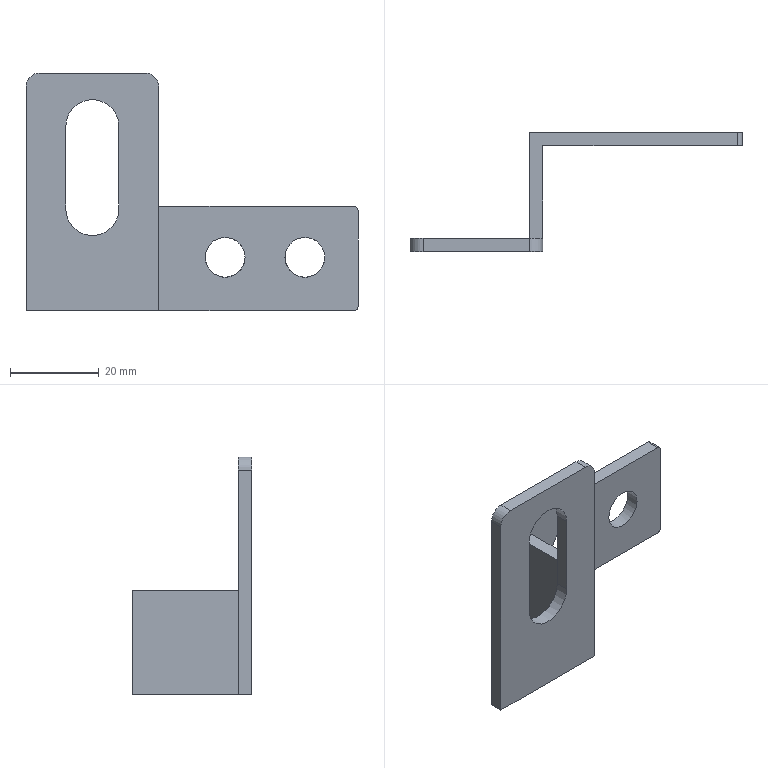Part | STEP file | 1 solid | 21 faces | box 75 x 27 x 53.7 mm | volume 8311 mm3 | plane 13 | cylinder 8 | commonest cylinder face diameters 2 x2 6 x2 9.002 x2 12 x2
STEP:
#1=CARTESIAN_POINT('',(-114.,-189.5,25.));
#2=VERTEX_POINT('',#1);
#3=CARTESIAN_POINT('',(-138.,-189.5,25.));
#4=VERTEX_POINT('',#3);
#5=CARTESIAN_POINT('',(-119.525,-189.5,25.));
#6=DIRECTION('',(-1.,0.,0.));
#7=VECTOR('',#6,1.);
#8=LINE('',#5,#7);
#9=EDGE_CURVE('',#2,#4,#8,.T.);
#10=ORIENTED_EDGE('',*,*,#9,.F.);
#11=CARTESIAN_POINT('',(-114.,-186.5,25.));
#12=VERTEX_POINT('',#11);
#13=CARTESIAN_POINT('',(-114.,-189.5,25.));
#14=DIRECTION('',(0.,1.,0.));
#15=VECTOR('',#14,1.);
#16=LINE('',#13,#15);
#17=EDGE_CURVE('',#2,#12,#16,.T.);
#18=ORIENTED_EDGE('',*,*,#17,.T.);
#19=CARTESIAN_POINT('',(-138.,-186.5,25.));
#20=VERTEX_POINT('',#19);
#21=CARTESIAN_POINT('',(-119.525,-186.5,25.));
#22=DIRECTION('',(1.,0.,0.));
#23=VECTOR('',#22,1.);
#24=LINE('',#21,#23);
#25=EDGE_CURVE('',#20,#12,#24,.T.);
#26=ORIENTED_EDGE('',*,*,#25,.F.);
#27=CARTESIAN_POINT('',(-138.,-182.452,25.));
#28=DIRECTION('',(0.,-1.,0.));
#29=VECTOR('',#28,1.);
#30=LINE('',#27,#29);
#31=EDGE_CURVE('',#20,#4,#30,.T.);
#32=ORIENTED_EDGE('',*,*,#31,.T.);
#33=EDGE_LOOP('',(#10,#18,#26,#32));
#34=FACE_OUTER_BOUND('',#33,.T.);
#35=CARTESIAN_POINT('',(-100.412,-182.452,25.));
#36=DIRECTION('',(0.,0.,1.));
#37=DIRECTION('',(-1.,0.,0.));
#38=AXIS2_PLACEMENT_3D('',#35,#36,#37);
#39=PLANE('',#38);
#40=ADVANCED_FACE('',(#34),#39,.T.);
#41=CARTESIAN_POINT('',(-111.,-186.5,22.));
#42=VERTEX_POINT('',#41);
#43=CARTESIAN_POINT('',(-114.,-186.5,22.));
#44=DIRECTION('',(0.,1.,0.));
#45=DIRECTION('',(0.,0.,-1.));
#46=AXIS2_PLACEMENT_3D('',#43,#44,#45);
#47=CIRCLE('',#46,3.);
#48=EDGE_CURVE('',#12,#42,#47,.T.);
#49=ORIENTED_EDGE('',*,*,#48,.F.);
#50=ORIENTED_EDGE('',*,*,#17,.F.);
#51=CARTESIAN_POINT('',(-111.,-189.5,22.));
#52=VERTEX_POINT('',#51);
#53=CARTESIAN_POINT('',(-114.,-189.5,22.));
#54=DIRECTION('',(0.,-1.,0.));
#55=DIRECTION('',(0.,0.,-1.));
#56=AXIS2_PLACEMENT_3D('',#53,#54,#55);
#57=CIRCLE('',#56,3.);
#58=EDGE_CURVE('',#52,#2,#57,.T.);
#59=ORIENTED_EDGE('',*,*,#58,.F.);
#60=CARTESIAN_POINT('',(-111.,-186.5,22.));
#61=DIRECTION('',(0.,-1.,0.));
#62=VECTOR('',#61,1.);
#63=LINE('',#60,#62);
#64=EDGE_CURVE('',#42,#52,#63,.T.);
#65=ORIENTED_EDGE('',*,*,#64,.F.);
#66=EDGE_LOOP('',(#49,#50,#59,#65));
#67=FACE_OUTER_BOUND('',#66,.T.);
#68=CARTESIAN_POINT('',(-114.,-182.452,22.));
#69=DIRECTION('',(0.,1.,0.));
#70=DIRECTION('',(0.,0.,1.));
#71=AXIS2_PLACEMENT_3D('',#68,#69,#70);
#72=CYLINDRICAL_SURFACE('',#71,3.);
#73=ADVANCED_FACE('',(#67),#72,.T.);
#74=CARTESIAN_POINT('',(-141.,-186.5,22.));
#75=VERTEX_POINT('',#74);
#76=CARTESIAN_POINT('',(-138.,-186.5,22.));
#77=DIRECTION('',(0.,1.,0.));
#78=DIRECTION('',(0.,0.,-1.));
#79=AXIS2_PLACEMENT_3D('',#76,#77,#78);
#80=CIRCLE('',#79,3.);
#81=EDGE_CURVE('',#75,#20,#80,.T.);
#82=ORIENTED_EDGE('',*,*,#81,.F.);
#83=CARTESIAN_POINT('',(-141.,-189.5,22.));
#84=VERTEX_POINT('',#83);
#85=CARTESIAN_POINT('',(-141.,-187.452,22.));
#86=DIRECTION('',(0.,1.,0.));
#87=VECTOR('',#86,1.);
#88=LINE('',#85,#87);
#89=EDGE_CURVE('',#84,#75,#88,.T.);
#90=ORIENTED_EDGE('',*,*,#89,.F.);
#91=CARTESIAN_POINT('',(-138.,-189.5,22.));
#92=DIRECTION('',(0.,-1.,0.));
#93=DIRECTION('',(0.,0.,-1.));
#94=AXIS2_PLACEMENT_3D('',#91,#92,#93);
#95=CIRCLE('',#94,3.);
#96=EDGE_CURVE('',#4,#84,#95,.T.);
#97=ORIENTED_EDGE('',*,*,#96,.F.);
#98=ORIENTED_EDGE('',*,*,#31,.F.);
#99=EDGE_LOOP('',(#82,#90,#97,#98));
#100=FACE_OUTER_BOUND('',#99,.T.);
#101=CARTESIAN_POINT('',(-138.,-187.452,22.));
#102=DIRECTION('',(0.,-1.,0.));
#103=DIRECTION('',(0.,0.,-1.));
#104=AXIS2_PLACEMENT_3D('',#101,#102,#103);
#105=CYLINDRICAL_SURFACE('',#104,3.);
#106=ADVANCED_FACE('',(#100),#105,.T.);
#107=CARTESIAN_POINT('',(-132.,-189.5,-5.7));
#108=VERTEX_POINT('',#107);
#109=CARTESIAN_POINT('',(-132.,-186.5,-5.7));
#110=VERTEX_POINT('',#109);
#111=CARTESIAN_POINT('',(-132.,-89.5,-5.7));
#112=DIRECTION('',(0.,1.,0.));
#113=VECTOR('',#112,1.);
#114=LINE('',#111,#113);
#115=EDGE_CURVE('',#108,#110,#114,.T.);
#116=ORIENTED_EDGE('',*,*,#115,.F.);
#117=CARTESIAN_POINT('',(-120.,-189.5,-5.7));
#118=VERTEX_POINT('',#117);
#119=CARTESIAN_POINT('',(-126.,-189.5,-5.7));
#120=DIRECTION('',(0.,1.,0.));
#121=DIRECTION('',(0.,0.,1.));
#122=AXIS2_PLACEMENT_3D('',#119,#120,#121);
#123=CIRCLE('',#122,6.);
#124=EDGE_CURVE('',#118,#108,#123,.T.);
#125=ORIENTED_EDGE('',*,*,#124,.F.);
#126=CARTESIAN_POINT('',(-120.,-186.5,-5.7));
#127=VERTEX_POINT('',#126);
#128=CARTESIAN_POINT('',(-120.,-89.5,-5.7));
#129=DIRECTION('',(0.,-1.,0.));
#130=VECTOR('',#129,1.);
#131=LINE('',#128,#130);
#132=EDGE_CURVE('',#127,#118,#131,.T.);
#133=ORIENTED_EDGE('',*,*,#132,.F.);
#134=CARTESIAN_POINT('',(-126.,-186.5,-5.7));
#135=DIRECTION('',(0.,-1.,0.));
#136=DIRECTION('',(0.,0.,-1.));
#137=AXIS2_PLACEMENT_3D('',#134,#135,#136);
#138=CIRCLE('',#137,6.);
#139=EDGE_CURVE('',#110,#127,#138,.T.);
#140=ORIENTED_EDGE('',*,*,#139,.F.);
#141=EDGE_LOOP('',(#116,#125,#133,#140));
#142=FACE_OUTER_BOUND('',#141,.T.);
#143=CARTESIAN_POINT('',(-126.,-89.5,-5.7));
#144=DIRECTION('',(0.,-1.,0.));
#145=DIRECTION('',(0.,0.,-1.));
#146=AXIS2_PLACEMENT_3D('',#143,#144,#145);
#147=CYLINDRICAL_SURFACE('',#146,6.);
#148=ADVANCED_FACE('',(#142),#147,.F.);
#149=CARTESIAN_POINT('',(-120.,-186.5,13.));
#150=VERTEX_POINT('',#149);
#151=CARTESIAN_POINT('',(-120.,-186.5,-18.1));
#152=DIRECTION('',(0.,0.,-1.));
#153=VECTOR('',#152,1.);
#154=LINE('',#151,#153);
#155=EDGE_CURVE('',#150,#127,#154,.T.);
#156=ORIENTED_EDGE('',*,*,#155,.T.);
#157=ORIENTED_EDGE('',*,*,#132,.T.);
#158=CARTESIAN_POINT('',(-120.,-189.5,13.));
#159=VERTEX_POINT('',#158);
#160=CARTESIAN_POINT('',(-120.,-189.5,-18.1));
#161=DIRECTION('',(0.,0.,-1.));
#162=VECTOR('',#161,1.);
#163=LINE('',#160,#162);
#164=EDGE_CURVE('',#159,#118,#163,.T.);
#165=ORIENTED_EDGE('',*,*,#164,.F.);
#166=CARTESIAN_POINT('',(-120.,-89.5,13.));
#167=DIRECTION('',(0.,1.,0.));
#168=VECTOR('',#167,1.);
#169=LINE('',#166,#168);
#170=EDGE_CURVE('',#159,#150,#169,.T.);
#171=ORIENTED_EDGE('',*,*,#170,.T.);
#172=EDGE_LOOP('',(#156,#157,#165,#171));
#173=FACE_OUTER_BOUND('',#172,.T.);
#174=CARTESIAN_POINT('',(-120.,-902.5,7.));
#175=DIRECTION('',(1.,0.,0.));
#176=DIRECTION('',(0.,0.,1.));
#177=AXIS2_PLACEMENT_3D('',#174,#175,#176);
#178=PLANE('',#177);
#179=ADVANCED_FACE('',(#173),#178,.F.);
#180=CARTESIAN_POINT('',(-132.,-186.5,13.));
#181=VERTEX_POINT('',#180);
#182=CARTESIAN_POINT('',(-126.,-186.5,13.));
#183=DIRECTION('',(0.,-1.,0.));
#184=DIRECTION('',(0.,0.,-1.));
#185=AXIS2_PLACEMENT_3D('',#182,#183,#184);
#186=CIRCLE('',#185,6.);
#187=EDGE_CURVE('',#150,#181,#186,.T.);
#188=ORIENTED_EDGE('',*,*,#187,.F.);
#189=ORIENTED_EDGE('',*,*,#170,.F.);
#190=CARTESIAN_POINT('',(-132.,-189.5,13.));
#191=VERTEX_POINT('',#190);
#192=CARTESIAN_POINT('',(-126.,-189.5,13.));
#193=DIRECTION('',(0.,1.,0.));
#194=DIRECTION('',(0.,0.,1.));
#195=AXIS2_PLACEMENT_3D('',#192,#193,#194);
#196=CIRCLE('',#195,6.);
#197=EDGE_CURVE('',#191,#159,#196,.T.);
#198=ORIENTED_EDGE('',*,*,#197,.F.);
#199=CARTESIAN_POINT('',(-132.,-89.5,13.));
#200=DIRECTION('',(0.,-1.,0.));
#201=VECTOR('',#200,1.);
#202=LINE('',#199,#201);
#203=EDGE_CURVE('',#181,#191,#202,.T.);
#204=ORIENTED_EDGE('',*,*,#203,.F.);
#205=EDGE_LOOP('',(#188,#189,#198,#204));
#206=FACE_OUTER_BOUND('',#205,.T.);
#207=CARTESIAN_POINT('',(-126.,-89.5,13.));
#208=DIRECTION('',(0.,-1.,0.));
#209=DIRECTION('',(0.,0.,-1.));
#210=AXIS2_PLACEMENT_3D('',#207,#208,#209);
#211=CYLINDRICAL_SURFACE('',#210,6.);
#212=ADVANCED_FACE('',(#206),#211,.F.);
#213=CARTESIAN_POINT('',(-132.,-186.5,-18.1));
#214=DIRECTION('',(0.,0.,-1.));
#215=VECTOR('',#214,1.);
#216=LINE('',#213,#215);
#217=EDGE_CURVE('',#181,#110,#216,.T.);
#218=ORIENTED_EDGE('',*,*,#217,.F.);
#219=ORIENTED_EDGE('',*,*,#203,.T.);
#220=CARTESIAN_POINT('',(-132.,-189.5,-18.1));
#221=DIRECTION('',(0.,0.,-1.));
#222=VECTOR('',#221,1.);
#223=LINE('',#220,#222);
#224=EDGE_CURVE('',#191,#108,#223,.T.);
#225=ORIENTED_EDGE('',*,*,#224,.T.);
#226=ORIENTED_EDGE('',*,*,#115,.T.);
#227=EDGE_LOOP('',(#218,#219,#225,#226));
#228=FACE_OUTER_BOUND('',#227,.T.);
#229=CARTESIAN_POINT('',(-132.,-902.5,13.));
#230=DIRECTION('',(-1.,0.,0.));
#231=DIRECTION('',(0.,0.,-1.));
#232=AXIS2_PLACEMENT_3D('',#229,#230,#231);
#233=PLANE('',#232);
#234=ADVANCED_FACE('',(#228),#233,.F.);
#235=CARTESIAN_POINT('',(-111.,-189.5,-28.7));
#236=VERTEX_POINT('',#235);
#237=CARTESIAN_POINT('',(-111.,-189.5,-18.1));
#238=DIRECTION('',(0.,0.,1.));
#239=VECTOR('',#238,1.);
#240=LINE('',#237,#239);
#241=EDGE_CURVE('',#236,#52,#240,.T.);
#242=ORIENTED_EDGE('',*,*,#241,.F.);
#243=CARTESIAN_POINT('',(-111.,-165.5,-28.7));
#244=VERTEX_POINT('',#243);
#245=CARTESIAN_POINT('',(-111.,-168.,-28.7));
#246=DIRECTION('',(0.,-1.,0.));
#247=VECTOR('',#246,1.);
#248=LINE('',#245,#247);
#249=EDGE_CURVE('',#244,#236,#248,.T.);
#250=ORIENTED_EDGE('',*,*,#249,.F.);
#251=CARTESIAN_POINT('',(-111.,-165.5,-5.1));
#252=VERTEX_POINT('',#251);
#253=CARTESIAN_POINT('',(-111.,-165.5,-32.7));
#254=DIRECTION('',(0.,0.,1.));
#255=VECTOR('',#254,1.);
#256=LINE('',#253,#255);
#257=EDGE_CURVE('',#244,#252,#256,.T.);
#258=ORIENTED_EDGE('',*,*,#257,.T.);
#259=CARTESIAN_POINT('',(-111.,-186.5,-5.1));
#260=VERTEX_POINT('',#259);
#261=CARTESIAN_POINT('',(-111.,-168.,-5.1));
#262=DIRECTION('',(0.,1.,0.));
#263=VECTOR('',#262,1.);
#264=LINE('',#261,#263);
#265=EDGE_CURVE('',#260,#252,#264,.T.);
#266=ORIENTED_EDGE('',*,*,#265,.F.);
#267=CARTESIAN_POINT('',(-111.,-186.5,-18.1));
#268=DIRECTION('',(0.,0.,1.));
#269=VECTOR('',#268,1.);
#270=LINE('',#267,#269);
#271=EDGE_CURVE('',#260,#42,#270,.T.);
#272=ORIENTED_EDGE('',*,*,#271,.T.);
#273=ORIENTED_EDGE('',*,*,#64,.T.);
#274=EDGE_LOOP('',(#242,#250,#258,#266,#272,#273));
#275=FACE_OUTER_BOUND('',#274,.T.);
#276=CARTESIAN_POINT('',(-111.,-185.,6.));
#277=DIRECTION('',(-1.,0.,0.));
#278=DIRECTION('',(0.,0.,-1.));
#279=AXIS2_PLACEMENT_3D('',#276,#277,#278);
#280=PLANE('',#279);
#281=ADVANCED_FACE('',(#275),#280,.F.);
#282=ORIENTED_EDGE('',*,*,#224,.F.);
#283=ORIENTED_EDGE('',*,*,#197,.T.);
#284=ORIENTED_EDGE('',*,*,#164,.T.);
#285=ORIENTED_EDGE('',*,*,#124,.T.);
#286=EDGE_LOOP('',(#282,#283,#284,#285));
#287=FACE_BOUND('',#286,.T.);
#288=CARTESIAN_POINT('',(-141.,-189.5,-28.7));
#289=VERTEX_POINT('',#288);
#290=CARTESIAN_POINT('',(-96.,-189.5,-28.7));
#291=DIRECTION('',(1.,0.,0.));
#292=VECTOR('',#291,1.);
#293=LINE('',#290,#292);
#294=EDGE_CURVE('',#289,#236,#293,.T.);
#295=ORIENTED_EDGE('',*,*,#294,.T.);
#296=ORIENTED_EDGE('',*,*,#241,.T.);
#297=ORIENTED_EDGE('',*,*,#58,.T.);
#298=ORIENTED_EDGE('',*,*,#9,.T.);
#299=ORIENTED_EDGE('',*,*,#96,.T.);
#300=CARTESIAN_POINT('',(-141.,-189.5,-20.));
#301=DIRECTION('',(0.,0.,1.));
#302=VECTOR('',#301,1.);
#303=LINE('',#300,#302);
#304=EDGE_CURVE('',#289,#84,#303,.T.);
#305=ORIENTED_EDGE('',*,*,#304,.F.);
#306=EDGE_LOOP('',(#295,#296,#297,#298,#299,#305));
#307=FACE_BOUND('',#306,.T.);
#308=CARTESIAN_POINT('',(-96.,-189.5,-20.));
#309=DIRECTION('',(0.,1.,0.));
#310=DIRECTION('',(0.,0.,-1.));
#311=AXIS2_PLACEMENT_3D('',#308,#309,#310);
#312=PLANE('',#311);
#313=ADVANCED_FACE('',(#287,#307),#312,.F.);
#314=ORIENTED_EDGE('',*,*,#89,.T.);
#315=CARTESIAN_POINT('',(-141.,-186.5,-28.7));
#316=VERTEX_POINT('',#315);
#317=CARTESIAN_POINT('',(-141.,-186.5,-18.1));
#318=DIRECTION('',(0.,0.,-1.));
#319=VECTOR('',#318,1.);
#320=LINE('',#317,#319);
#321=EDGE_CURVE('',#75,#316,#320,.T.);
#322=ORIENTED_EDGE('',*,*,#321,.T.);
#323=CARTESIAN_POINT('',(-141.,-141.153,-28.7));
#324=DIRECTION('',(0.,-1.,0.));
#325=VECTOR('',#324,1.);
#326=LINE('',#323,#325);
#327=EDGE_CURVE('',#316,#289,#326,.T.);
#328=ORIENTED_EDGE('',*,*,#327,.T.);
#329=ORIENTED_EDGE('',*,*,#304,.T.);
#330=EDGE_LOOP('',(#314,#322,#328,#329));
#331=FACE_OUTER_BOUND('',#330,.T.);
#332=CARTESIAN_POINT('',(-141.,-187.452,-3.6));
#333=DIRECTION('',(-1.,0.,0.));
#334=DIRECTION('',(0.,0.,-1.));
#335=AXIS2_PLACEMENT_3D('',#332,#333,#334);
#336=PLANE('',#335);
#337=ADVANCED_FACE('',(#331),#336,.T.);
#338=ORIENTED_EDGE('',*,*,#217,.T.);
#339=ORIENTED_EDGE('',*,*,#139,.T.);
#340=ORIENTED_EDGE('',*,*,#155,.F.);
#341=ORIENTED_EDGE('',*,*,#187,.T.);
#342=EDGE_LOOP('',(#338,#339,#340,#341));
#343=FACE_BOUND('',#342,.T.);
#344=ORIENTED_EDGE('',*,*,#81,.T.);
#345=ORIENTED_EDGE('',*,*,#25,.T.);
#346=ORIENTED_EDGE('',*,*,#48,.T.);
#347=ORIENTED_EDGE('',*,*,#271,.F.);
#348=CARTESIAN_POINT('',(-114.,-186.5,-5.1));
#349=VERTEX_POINT('',#348);
#350=CARTESIAN_POINT('',(-94.5,-186.5,-5.1));
#351=DIRECTION('',(1.,0.,0.));
#352=VECTOR('',#351,1.);
#353=LINE('',#350,#352);
#354=EDGE_CURVE('',#349,#260,#353,.T.);
#355=ORIENTED_EDGE('',*,*,#354,.F.);
#356=CARTESIAN_POINT('',(-114.,-186.5,-28.7));
#357=VERTEX_POINT('',#356);
#358=CARTESIAN_POINT('',(-114.,-186.5,-30.8));
#359=DIRECTION('',(0.,0.,1.));
#360=VECTOR('',#359,1.);
#361=LINE('',#358,#360);
#362=EDGE_CURVE('',#357,#349,#361,.T.);
#363=ORIENTED_EDGE('',*,*,#362,.F.);
#364=CARTESIAN_POINT('',(-132.475,-186.5,-28.7));
#365=DIRECTION('',(-1.,0.,0.));
#366=VECTOR('',#365,1.);
#367=LINE('',#364,#366);
#368=EDGE_CURVE('',#357,#316,#367,.T.);
#369=ORIENTED_EDGE('',*,*,#368,.T.);
#370=ORIENTED_EDGE('',*,*,#321,.F.);
#371=EDGE_LOOP('',(#344,#345,#346,#347,#355,#363,#369,#370));
#372=FACE_BOUND('',#371,.T.);
#373=CARTESIAN_POINT('',(-132.475,-186.5,-18.1));
#374=DIRECTION('',(0.,-1.,0.));
#375=DIRECTION('',(0.,0.,1.));
#376=AXIS2_PLACEMENT_3D('',#373,#374,#375);
#377=PLANE('',#376);
#378=ADVANCED_FACE('',(#343,#372),#377,.F.);
#379=CARTESIAN_POINT('',(-96.,-162.5,-21.101));
#380=VERTEX_POINT('',#379);
#381=CARTESIAN_POINT('',(-96.,-162.5,-16.6));
#382=DIRECTION('',(0.,-1.,0.));
#383=DIRECTION('',(0.,0.,-1.));
#384=AXIS2_PLACEMENT_3D('',#381,#382,#383);
#385=CIRCLE('',#384,4.501);
#386=EDGE_CURVE('',#380,#380,#385,.T.);
#387=ORIENTED_EDGE('',*,*,#386,.F.);
#388=EDGE_LOOP('',(#387));
#389=FACE_BOUND('',#388,.T.);
#390=CARTESIAN_POINT('',(-91.499,-165.5,-16.6));
#391=VERTEX_POINT('',#390);
#392=CARTESIAN_POINT('',(-96.,-165.5,-16.6));
#393=DIRECTION('',(0.,-1.,0.));
#394=DIRECTION('',(1.,0.,0.));
#395=AXIS2_PLACEMENT_3D('',#392,#393,#394);
#396=CIRCLE('',#395,4.501);
#397=EDGE_CURVE('',#391,#391,#396,.T.);
#398=ORIENTED_EDGE('',*,*,#397,.T.);
#399=EDGE_LOOP('',(#398));
#400=FACE_BOUND('',#399,.T.);
#401=CARTESIAN_POINT('',(-96.,-165.5,-16.6));
#402=DIRECTION('',(0.,1.,0.));
#403=DIRECTION('',(0.,0.,1.));
#404=AXIS2_PLACEMENT_3D('',#401,#402,#403);
#405=CYLINDRICAL_SURFACE('',#404,4.501);
#406=ADVANCED_FACE('',(#389,#400),#405,.F.);
#407=CARTESIAN_POINT('',(-67.,-165.5,-5.1));
#408=VERTEX_POINT('',#407);
#409=CARTESIAN_POINT('',(-112.5,-165.5,-5.1));
#410=DIRECTION('',(1.,0.,0.));
#411=VECTOR('',#410,1.);
#412=LINE('',#409,#411);
#413=EDGE_CURVE('',#252,#408,#412,.T.);
#414=ORIENTED_EDGE('',*,*,#413,.T.);
#415=CARTESIAN_POINT('',(-67.,-162.5,-5.1));
#416=VERTEX_POINT('',#415);
#417=CARTESIAN_POINT('',(-67.,-174.,-5.1));
#418=DIRECTION('',(0.,-1.,0.));
#419=VECTOR('',#418,1.);
#420=LINE('',#417,#419);
#421=EDGE_CURVE('',#416,#408,#420,.T.);
#422=ORIENTED_EDGE('',*,*,#421,.F.);
#423=CARTESIAN_POINT('',(-114.,-162.5,-5.1));
#424=VERTEX_POINT('',#423);
#425=CARTESIAN_POINT('',(-112.5,-162.5,-5.1));
#426=DIRECTION('',(-1.,0.,0.));
#427=VECTOR('',#426,1.);
#428=LINE('',#425,#427);
#429=EDGE_CURVE('',#416,#424,#428,.T.);
#430=ORIENTED_EDGE('',*,*,#429,.T.);
#431=CARTESIAN_POINT('',(-114.,-156.7,-5.1));
#432=DIRECTION('',(0.,1.,0.));
#433=VECTOR('',#432,1.);
#434=LINE('',#431,#433);
#435=EDGE_CURVE('',#349,#424,#434,.T.);
#436=ORIENTED_EDGE('',*,*,#435,.F.);
#437=ORIENTED_EDGE('',*,*,#354,.T.);
#438=ORIENTED_EDGE('',*,*,#265,.T.);
#439=EDGE_LOOP('',(#414,#422,#430,#436,#437,#438));
#440=FACE_OUTER_BOUND('',#439,.T.);
#441=CARTESIAN_POINT('',(-94.5,-156.7,-5.1));
#442=DIRECTION('',(0.,0.,-1.));
#443=DIRECTION('',(1.,0.,0.));
#444=AXIS2_PLACEMENT_3D('',#441,#442,#443);
#445=PLANE('',#444);
#446=ADVANCED_FACE('',(#440),#445,.F.);
#447=CARTESIAN_POINT('',(-66.,-162.5,-6.1));
#448=VERTEX_POINT('',#447);
#449=CARTESIAN_POINT('',(-67.,-162.5,-6.1));
#450=DIRECTION('',(0.,-1.,0.));
#451=DIRECTION('',(0.,0.,-1.));
#452=AXIS2_PLACEMENT_3D('',#449,#450,#451);
#453=CIRCLE('',#452,1.);
#454=EDGE_CURVE('',#448,#416,#453,.T.);
#455=ORIENTED_EDGE('',*,*,#454,.T.);
#456=ORIENTED_EDGE('',*,*,#421,.T.);
#457=CARTESIAN_POINT('',(-66.,-165.5,-6.1));
#458=VERTEX_POINT('',#457);
#459=CARTESIAN_POINT('',(-67.,-165.5,-6.1));
#460=DIRECTION('',(0.,1.,0.));
#461=DIRECTION('',(-1.,0.,0.));
#462=AXIS2_PLACEMENT_3D('',#459,#460,#461);
#463=CIRCLE('',#462,1.);
#464=EDGE_CURVE('',#408,#458,#463,.T.);
#465=ORIENTED_EDGE('',*,*,#464,.T.);
#466=CARTESIAN_POINT('',(-66.,-163.5,-6.1));
#467=DIRECTION('',(0.,1.,0.));
#468=VECTOR('',#467,1.);
#469=LINE('',#466,#468);
#470=EDGE_CURVE('',#458,#448,#469,.T.);
#471=ORIENTED_EDGE('',*,*,#470,.T.);
#472=EDGE_LOOP('',(#455,#456,#465,#471));
#473=FACE_OUTER_BOUND('',#472,.T.);
#474=CARTESIAN_POINT('',(-67.,-174.,-6.1));
#475=DIRECTION('',(0.,1.,0.));
#476=DIRECTION('',(0.,0.,1.));
#477=AXIS2_PLACEMENT_3D('',#474,#475,#476);
#478=CYLINDRICAL_SURFACE('',#477,1.);
#479=ADVANCED_FACE('',(#473),#478,.T.);
#480=CARTESIAN_POINT('',(-66.,-165.5,-27.7));
#481=VERTEX_POINT('',#480);
#482=CARTESIAN_POINT('',(-66.,-165.5,-32.7));
#483=DIRECTION('',(0.,0.,1.));
#484=VECTOR('',#483,1.);
#485=LINE('',#482,#484);
#486=EDGE_CURVE('',#481,#458,#485,.T.);
#487=ORIENTED_EDGE('',*,*,#486,.F.);
#488=CARTESIAN_POINT('',(-66.,-162.5,-27.7));
#489=VERTEX_POINT('',#488);
#490=CARTESIAN_POINT('',(-66.,-163.5,-27.7));
#491=DIRECTION('',(0.,-1.,0.));
#492=VECTOR('',#491,1.);
#493=LINE('',#490,#492);
#494=EDGE_CURVE('',#489,#481,#493,.T.);
#495=ORIENTED_EDGE('',*,*,#494,.F.);
#496=CARTESIAN_POINT('',(-66.,-162.5,-30.8));
#497=DIRECTION('',(0.,0.,1.));
#498=VECTOR('',#497,1.);
#499=LINE('',#496,#498);
#500=EDGE_CURVE('',#489,#448,#499,.T.);
#501=ORIENTED_EDGE('',*,*,#500,.T.);
#502=ORIENTED_EDGE('',*,*,#470,.F.);
#503=EDGE_LOOP('',(#487,#495,#501,#502));
#504=FACE_OUTER_BOUND('',#503,.T.);
#505=CARTESIAN_POINT('',(-66.,-163.5,-32.7));
#506=DIRECTION('',(1.,0.,0.));
#507=DIRECTION('',(0.,0.,1.));
#508=AXIS2_PLACEMENT_3D('',#505,#506,#507);
#509=PLANE('',#508);
#510=ADVANCED_FACE('',(#504),#509,.T.);
#511=CARTESIAN_POINT('',(-67.,-162.5,-28.7));
#512=VERTEX_POINT('',#511);
#513=CARTESIAN_POINT('',(-67.,-162.5,-27.7));
#514=DIRECTION('',(0.,-1.,0.));
#515=DIRECTION('',(0.,0.,-1.));
#516=AXIS2_PLACEMENT_3D('',#513,#514,#515);
#517=CIRCLE('',#516,1.);
#518=EDGE_CURVE('',#512,#489,#517,.T.);
#519=ORIENTED_EDGE('',*,*,#518,.T.);
#520=ORIENTED_EDGE('',*,*,#494,.T.);
#521=CARTESIAN_POINT('',(-67.,-165.5,-28.7));
#522=VERTEX_POINT('',#521);
#523=CARTESIAN_POINT('',(-67.,-165.5,-27.7));
#524=DIRECTION('',(0.,1.,0.));
#525=DIRECTION('',(-1.,0.,0.));
#526=AXIS2_PLACEMENT_3D('',#523,#524,#525);
#527=CIRCLE('',#526,1.);
#528=EDGE_CURVE('',#481,#522,#527,.T.);
#529=ORIENTED_EDGE('',*,*,#528,.T.);
#530=CARTESIAN_POINT('',(-67.,-158.452,-28.7));
#531=DIRECTION('',(0.,1.,0.));
#532=VECTOR('',#531,1.);
#533=LINE('',#530,#532);
#534=EDGE_CURVE('',#522,#512,#533,.T.);
#535=ORIENTED_EDGE('',*,*,#534,.T.);
#536=EDGE_LOOP('',(#519,#520,#529,#535));
#537=FACE_OUTER_BOUND('',#536,.T.);
#538=CARTESIAN_POINT('',(-67.,-163.5,-27.7));
#539=DIRECTION('',(0.,-1.,0.));
#540=DIRECTION('',(0.,0.,-1.));
#541=AXIS2_PLACEMENT_3D('',#538,#539,#540);
#542=CYLINDRICAL_SURFACE('',#541,1.);
#543=ADVANCED_FACE('',(#537),#542,.T.);
#544=ORIENTED_EDGE('',*,*,#368,.F.);
#545=CARTESIAN_POINT('',(-114.,-162.5,-28.7));
#546=VERTEX_POINT('',#545);
#547=CARTESIAN_POINT('',(-114.,-141.153,-28.7));
#548=DIRECTION('',(0.,1.,0.));
#549=VECTOR('',#548,1.);
#550=LINE('',#547,#549);
#551=EDGE_CURVE('',#357,#546,#550,.T.);
#552=ORIENTED_EDGE('',*,*,#551,.T.);
#553=CARTESIAN_POINT('',(-150.475,-162.5,-28.7));
#554=DIRECTION('',(1.,0.,0.));
#555=VECTOR('',#554,1.);
#556=LINE('',#553,#555);
#557=EDGE_CURVE('',#546,#512,#556,.T.);
#558=ORIENTED_EDGE('',*,*,#557,.T.);
#559=ORIENTED_EDGE('',*,*,#534,.F.);
#560=CARTESIAN_POINT('',(-175.5,-165.5,-28.7));
#561=DIRECTION('',(-1.,0.,0.));
#562=VECTOR('',#561,1.);
#563=LINE('',#560,#562);
#564=EDGE_CURVE('',#522,#244,#563,.T.);
#565=ORIENTED_EDGE('',*,*,#564,.T.);
#566=ORIENTED_EDGE('',*,*,#249,.T.);
#567=ORIENTED_EDGE('',*,*,#294,.F.);
#568=ORIENTED_EDGE('',*,*,#327,.F.);
#569=EDGE_LOOP('',(#544,#552,#558,#559,#565,#566,#567,#568));
#570=FACE_OUTER_BOUND('',#569,.T.);
#571=CARTESIAN_POINT('',(-100.412,-141.153,-28.7));
#572=DIRECTION('',(0.,0.,-1.));
#573=DIRECTION('',(1.,0.,0.));
#574=AXIS2_PLACEMENT_3D('',#571,#572,#573);
#575=PLANE('',#574);
#576=ADVANCED_FACE('',(#570),#575,.T.);
#577=ORIENTED_EDGE('',*,*,#551,.F.);
#578=ORIENTED_EDGE('',*,*,#362,.T.);
#579=ORIENTED_EDGE('',*,*,#435,.T.);
#580=CARTESIAN_POINT('',(-114.,-162.5,-30.8));
#581=DIRECTION('',(0.,0.,-1.));
#582=VECTOR('',#581,1.);
#583=LINE('',#580,#582);
#584=EDGE_CURVE('',#424,#546,#583,.T.);
#585=ORIENTED_EDGE('',*,*,#584,.T.);
#586=EDGE_LOOP('',(#577,#578,#579,#585));
#587=FACE_OUTER_BOUND('',#586,.T.);
#588=CARTESIAN_POINT('',(-114.,-146.7,-19.2));
#589=DIRECTION('',(1.,0.,0.));
#590=DIRECTION('',(0.,0.,1.));
#591=AXIS2_PLACEMENT_3D('',#588,#589,#590);
#592=PLANE('',#591);
#593=ADVANCED_FACE('',(#587),#592,.F.);
#594=CARTESIAN_POINT('',(-78.,-162.5,-21.101));
#595=VERTEX_POINT('',#594);
#596=CARTESIAN_POINT('',(-78.,-162.5,-16.6));
#597=DIRECTION('',(0.,-1.,0.));
#598=DIRECTION('',(0.,0.,-1.));
#599=AXIS2_PLACEMENT_3D('',#596,#597,#598);
#600=CIRCLE('',#599,4.501);
#601=EDGE_CURVE('',#595,#595,#600,.T.);
#602=ORIENTED_EDGE('',*,*,#601,.T.);
#603=EDGE_LOOP('',(#602));
#604=FACE_BOUND('',#603,.T.);
#605=ORIENTED_EDGE('',*,*,#584,.F.);
#606=ORIENTED_EDGE('',*,*,#429,.F.);
#607=ORIENTED_EDGE('',*,*,#454,.F.);
#608=ORIENTED_EDGE('',*,*,#500,.F.);
#609=ORIENTED_EDGE('',*,*,#518,.F.);
#610=ORIENTED_EDGE('',*,*,#557,.F.);
#611=EDGE_LOOP('',(#605,#606,#607,#608,#609,#610));
#612=FACE_BOUND('',#611,.T.);
#613=ORIENTED_EDGE('',*,*,#386,.T.);
#614=EDGE_LOOP('',(#613));
#615=FACE_BOUND('',#614,.T.);
#616=CARTESIAN_POINT('',(-150.475,-162.5,-30.8));
#617=DIRECTION('',(0.,-1.,0.));
#618=DIRECTION('',(0.,0.,1.));
#619=AXIS2_PLACEMENT_3D('',#616,#617,#618);
#620=PLANE('',#619);
#621=ADVANCED_FACE('',(#604,#612,#615),#620,.F.);
#622=CARTESIAN_POINT('',(-73.499,-165.5,-16.6));
#623=VERTEX_POINT('',#622);
#624=CARTESIAN_POINT('',(-78.,-165.5,-16.6));
#625=DIRECTION('',(0.,1.,0.));
#626=DIRECTION('',(1.,0.,0.));
#627=AXIS2_PLACEMENT_3D('',#624,#625,#626);
#628=CIRCLE('',#627,4.501);
#629=EDGE_CURVE('',#623,#623,#628,.T.);
#630=ORIENTED_EDGE('',*,*,#629,.T.);
#631=EDGE_LOOP('',(#630));
#632=FACE_BOUND('',#631,.T.);
#633=ORIENTED_EDGE('',*,*,#397,.F.);
#634=EDGE_LOOP('',(#633));
#635=FACE_BOUND('',#634,.T.);
#636=ORIENTED_EDGE('',*,*,#564,.F.);
#637=ORIENTED_EDGE('',*,*,#528,.F.);
#638=ORIENTED_EDGE('',*,*,#486,.T.);
#639=ORIENTED_EDGE('',*,*,#464,.F.);
#640=ORIENTED_EDGE('',*,*,#413,.F.);
#641=ORIENTED_EDGE('',*,*,#257,.F.);
#642=EDGE_LOOP('',(#636,#637,#638,#639,#640,#641));
#643=FACE_BOUND('',#642,.T.);
#644=CARTESIAN_POINT('',(-175.5,-165.5,-32.7));
#645=DIRECTION('',(0.,-1.,0.));
#646=DIRECTION('',(0.,0.,-1.));
#647=AXIS2_PLACEMENT_3D('',#644,#645,#646);
#648=PLANE('',#647);
#649=ADVANCED_FACE('',(#632,#635,#643),#648,.T.);
#650=ORIENTED_EDGE('',*,*,#601,.F.);
#651=EDGE_LOOP('',(#650));
#652=FACE_BOUND('',#651,.T.);
#653=ORIENTED_EDGE('',*,*,#629,.F.);
#654=EDGE_LOOP('',(#653));
#655=FACE_BOUND('',#654,.T.);
#656=CARTESIAN_POINT('',(-78.,-165.5,-16.6));
#657=DIRECTION('',(0.,1.,0.));
#658=DIRECTION('',(0.,0.,1.));
#659=AXIS2_PLACEMENT_3D('',#656,#657,#658);
#660=CYLINDRICAL_SURFACE('',#659,4.501);
#661=ADVANCED_FACE('',(#652,#655),#660,.F.);
#662=CLOSED_SHELL('',(#40,#73,#106,#148,#179,#212,#234,#281,#313,#337,#378,#406,#446,#479,#510,#543,#576,#593,#621,#649,#661));
#663=MANIFOLD_SOLID_BREP('',#662);
#664=(LENGTH_UNIT()NAMED_UNIT(*)SI_UNIT(.MILLI.,.METRE.));
#665=UNCERTAINTY_MEASURE_WITH_UNIT(LENGTH_MEASURE(0.00002),#664,'','');
#666=(NAMED_UNIT(*)PLANE_ANGLE_UNIT()SI_UNIT($,.RADIAN.));
#667=PLANE_ANGLE_MEASURE_WITH_UNIT(PLANE_ANGLE_MEASURE(0.01745),#666);
#668=DIMENSIONAL_EXPONENTS(0.,0.,0.,0.,0.,0.,0.);
#669=(CONVERSION_BASED_UNIT('DEGREE',#667)NAMED_UNIT(#668)PLANE_ANGLE_UNIT());
#670=(NAMED_UNIT(*)SI_UNIT($,.STERADIAN.)SOLID_ANGLE_UNIT());
#671=(GEOMETRIC_REPRESENTATION_CONTEXT(3)GLOBAL_UNCERTAINTY_ASSIGNED_CONTEXT((#665))GLOBAL_UNIT_ASSIGNED_CONTEXT((#664,#669,#670))REPRESENTATION_CONTEXT('',''));
#672=ADVANCED_BREP_SHAPE_REPRESENTATION('',(#663),#671);